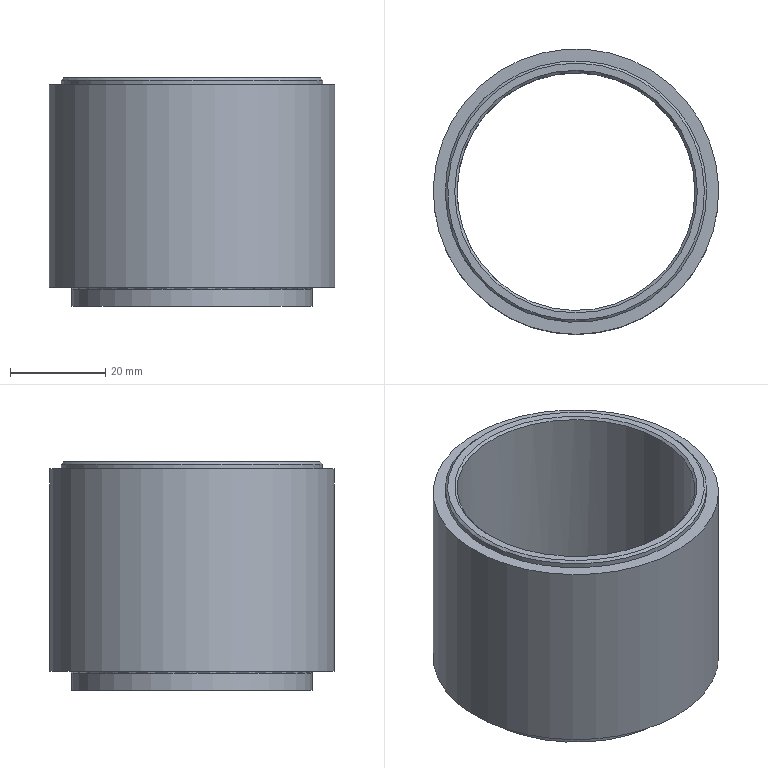Part | STEP file | 1 solid | 11 faces | box 60 x 60 x 48 mm | volume 37487 mm3 | plane 4 | cylinder 4 | cone 2 | torus 1 | commonest cylinder face diameters 50 x1 50.6 x1 54.97 x1 60 x1
STEP:
#1=CARTESIAN_POINT('',(23.383,13.5,31.69));
#2=VERTEX_POINT('',#1);
#3=CARTESIAN_POINT('',(0.,0.,31.69));
#4=DIRECTION('',(0.,0.,1.));
#5=DIRECTION('',(-0.866,0.5,0.));
#6=AXIS2_PLACEMENT_3D('',#3,#4,#5);
#7=CIRCLE('',#6,27.);
#8=EDGE_CURVE('',#2,#2,#7,.T.);
#9=ORIENTED_EDGE('',*,*,#8,.T.);
#10=EDGE_LOOP('',(#9));
#11=FACE_BOUND('',#10,.T.);
#12=CARTESIAN_POINT('',(22.084,12.75,31.69));
#13=VERTEX_POINT('',#12);
#14=CARTESIAN_POINT('',(0.,0.,31.69));
#15=DIRECTION('',(0.,0.,-1.));
#16=DIRECTION('',(0.,-1.,0.));
#17=AXIS2_PLACEMENT_3D('',#14,#15,#16);
#18=CIRCLE('',#17,25.5);
#19=EDGE_CURVE('',#13,#13,#18,.T.);
#20=ORIENTED_EDGE('',*,*,#19,.T.);
#21=EDGE_LOOP('',(#20));
#22=FACE_BOUND('',#21,.T.);
#23=CARTESIAN_POINT('',(0.,0.,31.69));
#24=DIRECTION('',(0.,0.,-1.));
#25=DIRECTION('',(0.,-1.,0.));
#26=AXIS2_PLACEMENT_3D('',#23,#24,#25);
#27=PLANE('',#26);
#28=ADVANCED_FACE('',(#11,#22),#27,.F.);
#29=CARTESIAN_POINT('',(23.803,13.742,31.205));
#30=VERTEX_POINT('',#29);
#31=CARTESIAN_POINT('',(-23.803,-13.742,31.205));
#32=VERTEX_POINT('',#31);
#33=CARTESIAN_POINT('',(0.,0.,31.205));
#34=DIRECTION('',(0.,0.,1.));
#35=DIRECTION('',(0.866,0.5,0.));
#36=AXIS2_PLACEMENT_3D('',#33,#34,#35);
#37=CIRCLE('',#36,27.485);
#38=EDGE_CURVE('',#30,#32,#37,.T.);
#39=ORIENTED_EDGE('',*,*,#38,.T.);
#40=CARTESIAN_POINT('',(0.,0.,31.205));
#41=DIRECTION('',(0.,0.,1.));
#42=DIRECTION('',(-0.866,-0.5,0.));
#43=AXIS2_PLACEMENT_3D('',#40,#41,#42);
#44=CIRCLE('',#43,27.485);
#45=EDGE_CURVE('',#32,#30,#44,.T.);
#46=ORIENTED_EDGE('',*,*,#45,.T.);
#47=EDGE_LOOP('',(#39,#46));
#48=FACE_BOUND('',#47,.T.);
#49=ORIENTED_EDGE('',*,*,#8,.F.);
#50=EDGE_LOOP('',(#49));
#51=FACE_OUTER_BOUND('',#50,.T.);
#52=CARTESIAN_POINT('',(0.,0.,31.447));
#53=DIRECTION('',(0.,0.,-1.));
#54=DIRECTION('',(0.866,0.5,0.));
#55=AXIS2_PLACEMENT_3D('',#52,#53,#54);
#56=CONICAL_SURFACE('',#55,27.243,0.7854);
#57=ADVANCED_FACE('',(#48,#51),#56,.T.);
#58=ORIENTED_EDGE('',*,*,#45,.F.);
#59=ORIENTED_EDGE('',*,*,#38,.F.);
#60=EDGE_LOOP('',(#58,#59));
#61=FACE_BOUND('',#60,.T.);
#62=CARTESIAN_POINT('',(-23.803,-13.742,30.19));
#63=VERTEX_POINT('',#62);
#64=CARTESIAN_POINT('',(0.,0.,30.19));
#65=DIRECTION('',(0.,0.,-1.));
#66=DIRECTION('',(0.866,0.5,0.));
#67=AXIS2_PLACEMENT_3D('',#64,#65,#66);
#68=CIRCLE('',#67,27.485);
#69=EDGE_CURVE('',#63,#63,#68,.T.);
#70=ORIENTED_EDGE('',*,*,#69,.F.);
#71=EDGE_LOOP('',(#70));
#72=FACE_OUTER_BOUND('',#71,.T.);
#73=CARTESIAN_POINT('',(0.,0.,30.115));
#74=DIRECTION('',(0.,0.,-1.));
#75=DIRECTION('',(-0.866,-0.5,0.));
#76=AXIS2_PLACEMENT_3D('',#73,#74,#75);
#77=CYLINDRICAL_SURFACE('',#76,27.485);
#78=ADVANCED_FACE('',(#61,#72),#77,.T.);
#79=CARTESIAN_POINT('',(25.981,15.,30.19));
#80=VERTEX_POINT('',#79);
#81=CARTESIAN_POINT('',(0.,0.,30.19));
#82=DIRECTION('',(0.,0.,1.));
#83=DIRECTION('',(0.866,0.5,0.));
#84=AXIS2_PLACEMENT_3D('',#81,#82,#83);
#85=CIRCLE('',#84,30.);
#86=EDGE_CURVE('',#80,#80,#85,.T.);
#87=ORIENTED_EDGE('',*,*,#86,.T.);
#88=EDGE_LOOP('',(#87));
#89=FACE_BOUND('',#88,.T.);
#90=ORIENTED_EDGE('',*,*,#69,.T.);
#91=EDGE_LOOP('',(#90));
#92=FACE_BOUND('',#91,.T.);
#93=CARTESIAN_POINT('',(0.,0.,30.19));
#94=DIRECTION('',(0.,0.,1.));
#95=DIRECTION('',(1.,0.,0.));
#96=AXIS2_PLACEMENT_3D('',#93,#94,#95);
#97=PLANE('',#96);
#98=ADVANCED_FACE('',(#89,#92),#97,.T.);
#99=ORIENTED_EDGE('',*,*,#86,.F.);
#100=EDGE_LOOP('',(#99));
#101=FACE_OUTER_BOUND('',#100,.T.);
#102=CARTESIAN_POINT('',(25.981,15.,-12.31));
#103=VERTEX_POINT('',#102);
#104=CARTESIAN_POINT('',(0.,0.,-12.31));
#105=DIRECTION('',(0.,0.,-1.));
#106=DIRECTION('',(0.866,0.5,0.));
#107=AXIS2_PLACEMENT_3D('',#104,#105,#106);
#108=CIRCLE('',#107,30.);
#109=EDGE_CURVE('',#103,#103,#108,.T.);
#110=ORIENTED_EDGE('',*,*,#109,.F.);
#111=EDGE_LOOP('',(#110));
#112=FACE_OUTER_BOUND('',#111,.T.);
#113=CARTESIAN_POINT('',(0.,0.,34.09));
#114=DIRECTION('',(0.,0.,1.));
#115=DIRECTION('',(-0.866,-0.5,0.));
#116=AXIS2_PLACEMENT_3D('',#113,#114,#115);
#117=CYLINDRICAL_SURFACE('',#116,30.);
#118=ADVANCED_FACE('',(#101,#112),#117,.T.);
#119=ORIENTED_EDGE('',*,*,#109,.T.);
#120=EDGE_LOOP('',(#119));
#121=FACE_BOUND('',#120,.T.);
#122=CARTESIAN_POINT('',(22.257,12.85,-12.31));
#123=VERTEX_POINT('',#122);
#124=CARTESIAN_POINT('',(0.,0.,-12.31));
#125=DIRECTION('',(0.,0.,1.));
#126=DIRECTION('',(0.866,0.5,0.));
#127=AXIS2_PLACEMENT_3D('',#124,#125,#126);
#128=CIRCLE('',#127,25.7);
#129=EDGE_CURVE('',#123,#123,#128,.T.);
#130=ORIENTED_EDGE('',*,*,#129,.T.);
#131=EDGE_LOOP('',(#130));
#132=FACE_BOUND('',#131,.T.);
#133=CARTESIAN_POINT('',(0.,0.,-12.31));
#134=DIRECTION('',(0.,0.,-1.));
#135=DIRECTION('',(0.,-1.,0.));
#136=AXIS2_PLACEMENT_3D('',#133,#134,#135);
#137=PLANE('',#136);
#138=ADVANCED_FACE('',(#121,#132),#137,.T.);
#139=ORIENTED_EDGE('',*,*,#129,.F.);
#140=EDGE_LOOP('',(#139));
#141=FACE_OUTER_BOUND('',#140,.T.);
#142=CARTESIAN_POINT('',(21.91,12.65,-12.71));
#143=VERTEX_POINT('',#142);
#144=CARTESIAN_POINT('',(-21.91,-12.65,-12.71));
#145=VERTEX_POINT('',#144);
#146=CARTESIAN_POINT('',(0.,0.,-12.71));
#147=DIRECTION('',(0.,0.,1.));
#148=DIRECTION('',(0.866,0.5,0.));
#149=AXIS2_PLACEMENT_3D('',#146,#147,#148);
#150=CIRCLE('',#149,25.3);
#151=EDGE_CURVE('',#143,#145,#150,.T.);
#152=ORIENTED_EDGE('',*,*,#151,.T.);
#153=CARTESIAN_POINT('',(0.,0.,-12.71));
#154=DIRECTION('',(0.,0.,1.));
#155=DIRECTION('',(-0.866,-0.5,0.));
#156=AXIS2_PLACEMENT_3D('',#153,#154,#155);
#157=CIRCLE('',#156,25.3);
#158=EDGE_CURVE('',#145,#143,#157,.T.);
#159=ORIENTED_EDGE('',*,*,#158,.T.);
#160=EDGE_LOOP('',(#152,#159));
#161=FACE_BOUND('',#160,.T.);
#162=CARTESIAN_POINT('',(0.,0.,-12.71));
#163=DIRECTION('',(0.,0.,-1.));
#164=DIRECTION('',(0.866,0.5,0.));
#165=AXIS2_PLACEMENT_3D('',#162,#163,#164);
#166=TOROIDAL_SURFACE('',#165,25.7,0.4);
#167=ADVANCED_FACE('',(#141,#161),#166,.F.);
#168=ORIENTED_EDGE('',*,*,#158,.F.);
#169=ORIENTED_EDGE('',*,*,#151,.F.);
#170=EDGE_LOOP('',(#168,#169));
#171=FACE_BOUND('',#170,.T.);
#172=CARTESIAN_POINT('',(-21.91,-12.65,-16.31));
#173=VERTEX_POINT('',#172);
#174=CARTESIAN_POINT('',(0.,0.,-16.31));
#175=DIRECTION('',(0.,0.,-1.));
#176=DIRECTION('',(0.866,0.5,0.));
#177=AXIS2_PLACEMENT_3D('',#174,#175,#176);
#178=CIRCLE('',#177,25.3);
#179=EDGE_CURVE('',#173,#173,#178,.T.);
#180=ORIENTED_EDGE('',*,*,#179,.F.);
#181=EDGE_LOOP('',(#180));
#182=FACE_OUTER_BOUND('',#181,.T.);
#183=CARTESIAN_POINT('',(0.,0.,34.09));
#184=DIRECTION('',(0.,0.,1.));
#185=DIRECTION('',(-0.866,-0.5,0.));
#186=AXIS2_PLACEMENT_3D('',#183,#184,#185);
#187=CYLINDRICAL_SURFACE('',#186,25.3);
#188=ADVANCED_FACE('',(#171,#182),#187,.T.);
#189=ORIENTED_EDGE('',*,*,#179,.T.);
#190=EDGE_LOOP('',(#189));
#191=FACE_BOUND('',#190,.T.);
#192=CARTESIAN_POINT('',(21.651,12.5,-16.31));
#193=VERTEX_POINT('',#192);
#194=CARTESIAN_POINT('',(0.,0.,-16.31));
#195=DIRECTION('',(0.,0.,1.));
#196=DIRECTION('',(0.866,0.5,0.));
#197=AXIS2_PLACEMENT_3D('',#194,#195,#196);
#198=CIRCLE('',#197,25.);
#199=EDGE_CURVE('',#193,#193,#198,.T.);
#200=ORIENTED_EDGE('',*,*,#199,.T.);
#201=EDGE_LOOP('',(#200));
#202=FACE_BOUND('',#201,.T.);
#203=CARTESIAN_POINT('',(0.,0.,-16.31));
#204=DIRECTION('',(0.,0.,-1.));
#205=DIRECTION('',(0.,-1.,0.));
#206=AXIS2_PLACEMENT_3D('',#203,#204,#205);
#207=PLANE('',#206);
#208=ADVANCED_FACE('',(#191,#202),#207,.T.);
#209=CARTESIAN_POINT('',(21.651,12.5,31.19));
#210=VERTEX_POINT('',#209);
#211=CARTESIAN_POINT('',(21.651,12.5,31.19));
#212=CARTESIAN_POINT('',(21.913,12.046,31.19));
#213=CARTESIAN_POINT('',(22.408,11.123,31.19));
#214=CARTESIAN_POINT('',(23.062,9.694,31.19));
#215=CARTESIAN_POINT('',(23.625,8.226,31.19));
#216=CARTESIAN_POINT('',(24.095,6.726,31.19));
#217=CARTESIAN_POINT('',(24.47,5.2,31.19));
#218=CARTESIAN_POINT('',(24.748,3.653,31.19));
#219=CARTESIAN_POINT('',(24.929,2.092,31.19));
#220=CARTESIAN_POINT('',(25.011,0.5219,31.19));
#221=CARTESIAN_POINT('',(24.994,-1.05,31.19));
#222=CARTESIAN_POINT('',(24.879,-2.617,31.19));
#223=CARTESIAN_POINT('',(24.666,-4.175,31.19));
#224=CARTESIAN_POINT('',(24.355,-5.715,31.19));
#225=CARTESIAN_POINT('',(23.948,-7.234,31.19));
#226=CARTESIAN_POINT('',(23.446,-8.723,31.19));
#227=CARTESIAN_POINT('',(22.852,-10.179,31.19));
#228=CARTESIAN_POINT('',(22.168,-11.594,31.19));
#229=CARTESIAN_POINT('',(21.396,-12.963,31.19));
#230=CARTESIAN_POINT('',(20.54,-14.281,31.19));
#231=CARTESIAN_POINT('',(19.602,-15.543,31.19));
#232=CARTESIAN_POINT('',(18.588,-16.743,31.19));
#233=CARTESIAN_POINT('',(17.499,-17.877,31.19));
#234=CARTESIAN_POINT('',(16.342,-18.941,31.19));
#235=CARTESIAN_POINT('',(15.12,-19.93,31.19));
#236=CARTESIAN_POINT('',(13.839,-20.84,31.19));
#237=CARTESIAN_POINT('',(12.503,-21.668,31.19));
#238=CARTESIAN_POINT('',(11.117,-22.41,31.19));
#239=CARTESIAN_POINT('',(9.688,-23.064,31.19));
#240=CARTESIAN_POINT('',(8.22,-23.627,31.19));
#241=CARTESIAN_POINT('',(6.72,-24.097,31.19));
#242=CARTESIAN_POINT('',(5.194,-24.471,31.19));
#243=CARTESIAN_POINT('',(3.647,-24.749,31.19));
#244=CARTESIAN_POINT('',(2.085,-24.929,31.19));
#245=CARTESIAN_POINT('',(0.5157,-25.011,31.19));
#246=CARTESIAN_POINT('',(-1.056,-24.994,31.19));
#247=CARTESIAN_POINT('',(-2.624,-24.879,31.19));
#248=CARTESIAN_POINT('',(-4.181,-24.665,31.19));
#249=CARTESIAN_POINT('',(-5.722,-24.353,31.19));
#250=CARTESIAN_POINT('',(-7.24,-23.946,31.19));
#251=CARTESIAN_POINT('',(-8.729,-23.444,31.19));
#252=CARTESIAN_POINT('',(-10.184,-22.85,31.19));
#253=CARTESIAN_POINT('',(-11.599,-22.165,31.19));
#254=CARTESIAN_POINT('',(-12.968,-21.393,31.19));
#255=CARTESIAN_POINT('',(-14.286,-20.536,31.19));
#256=CARTESIAN_POINT('',(-15.548,-19.598,31.19));
#257=CARTESIAN_POINT('',(-16.748,-18.583,31.19));
#258=CARTESIAN_POINT('',(-17.882,-17.495,31.19));
#259=CARTESIAN_POINT('',(-18.945,-16.337,31.19));
#260=CARTESIAN_POINT('',(-19.934,-15.115,31.19));
#261=CARTESIAN_POINT('',(-20.841,-13.837,31.19));
#262=CARTESIAN_POINT('',(-21.391,-12.95,31.19));
#263=CARTESIAN_POINT('',(-21.651,-12.5,31.19));
#264=CARTESIAN_POINT('',(-21.913,-12.046,31.19));
#265=CARTESIAN_POINT('',(-22.408,-11.123,31.19));
#266=CARTESIAN_POINT('',(-23.062,-9.694,31.19));
#267=CARTESIAN_POINT('',(-23.625,-8.226,31.19));
#268=CARTESIAN_POINT('',(-24.095,-6.726,31.19));
#269=CARTESIAN_POINT('',(-24.47,-5.2,31.19));
#270=CARTESIAN_POINT('',(-24.748,-3.653,31.19));
#271=CARTESIAN_POINT('',(-24.929,-2.092,31.19));
#272=CARTESIAN_POINT('',(-25.011,-0.5219,31.19));
#273=CARTESIAN_POINT('',(-24.994,1.05,31.19));
#274=CARTESIAN_POINT('',(-24.879,2.617,31.19));
#275=CARTESIAN_POINT('',(-24.666,4.175,31.19));
#276=CARTESIAN_POINT('',(-24.355,5.715,31.19));
#277=CARTESIAN_POINT('',(-23.948,7.234,31.19));
#278=CARTESIAN_POINT('',(-23.446,8.723,31.19));
#279=CARTESIAN_POINT('',(-22.852,10.179,31.19));
#280=CARTESIAN_POINT('',(-22.168,11.594,31.19));
#281=CARTESIAN_POINT('',(-21.396,12.963,31.19));
#282=CARTESIAN_POINT('',(-20.54,14.281,31.19));
#283=CARTESIAN_POINT('',(-19.602,15.543,31.19));
#284=CARTESIAN_POINT('',(-18.588,16.743,31.19));
#285=CARTESIAN_POINT('',(-17.499,17.877,31.19));
#286=CARTESIAN_POINT('',(-16.342,18.941,31.19));
#287=CARTESIAN_POINT('',(-15.12,19.93,31.19));
#288=CARTESIAN_POINT('',(-13.839,20.84,31.19));
#289=CARTESIAN_POINT('',(-12.503,21.668,31.19));
#290=CARTESIAN_POINT('',(-11.117,22.41,31.19));
#291=CARTESIAN_POINT('',(-9.688,23.064,31.19));
#292=CARTESIAN_POINT('',(-8.22,23.627,31.19));
#293=CARTESIAN_POINT('',(-6.72,24.097,31.19));
#294=CARTESIAN_POINT('',(-5.194,24.471,31.19));
#295=CARTESIAN_POINT('',(-3.647,24.749,31.19));
#296=CARTESIAN_POINT('',(-2.085,24.929,31.19));
#297=CARTESIAN_POINT('',(-0.5157,25.011,31.19));
#298=CARTESIAN_POINT('',(1.056,24.994,31.19));
#299=CARTESIAN_POINT('',(2.624,24.879,31.19));
#300=CARTESIAN_POINT('',(4.181,24.665,31.19));
#301=CARTESIAN_POINT('',(5.722,24.353,31.19));
#302=CARTESIAN_POINT('',(7.24,23.946,31.19));
#303=CARTESIAN_POINT('',(8.729,23.444,31.19));
#304=CARTESIAN_POINT('',(10.184,22.85,31.19));
#305=CARTESIAN_POINT('',(11.599,22.165,31.19));
#306=CARTESIAN_POINT('',(12.968,21.393,31.19));
#307=CARTESIAN_POINT('',(14.286,20.536,31.19));
#308=CARTESIAN_POINT('',(15.548,19.598,31.19));
#309=CARTESIAN_POINT('',(16.748,18.583,31.19));
#310=CARTESIAN_POINT('',(17.882,17.495,31.19));
#311=CARTESIAN_POINT('',(18.945,16.337,31.19));
#312=CARTESIAN_POINT('',(19.934,15.115,31.19));
#313=CARTESIAN_POINT('',(20.841,13.837,31.19));
#314=CARTESIAN_POINT('',(21.391,12.95,31.19));
#315=CARTESIAN_POINT('',(21.651,12.5,31.19));
#316=B_SPLINE_CURVE_WITH_KNOTS('',3,(#211,#212,#213,#214,#215,#216,#217,#218,#219,#220,#221,#222,#223,#224,#225,#226,#227,#228,#229,#230,#231,#232,#233,#234,#235,#236,#237,#238,#239,#240,#241,#242,#243,#244,#245,#246,#247,#248,#249,#250,#251,#252,#253,#254,#255,#256,#257,#258,#259,#260,#261,#262,#263,#264,#265,#266,#267,#268,#269,#270,#271,#272,#273,#274,#275,#276,#277,#278,#279,#280,#281,#282,#283,#284,#285,#286,#287,#288,#289,#290,#291,#292,#293,#294,#295,#296,#297,#298,#299,#300,#301,#302,#303,#304,#305,#306,#307,#308,#309,#310,#311,#312,#313,#314,#315),.UNSPECIFIED.,.T.,.F.,(4,1,1,1,1,1,1,1,1,1,1,1,1,1,1,1,1,1,1,1,1,1,1,1,1,1,1,1,1,1,1,1,1,1,1,1,1,1,1,1,1,1,1,1,1,1,1,1,1,1,3,1,1,1,1,1,1,1,1,1,1,1,1,1,1,1,1,1,1,1,1,1,1,1,1,1,1,1,1,1,1,1,1,1,1,1,1,1,1,1,1,1,1,1,1,1,1,1,1,1,4),(0.,0.01,0.02,0.03,0.04001,0.05001,0.06001,0.07001,0.08001,0.09001,0.1,0.11,0.12,0.13,0.14,0.15,0.16,0.17,0.18,0.19,0.2,0.21,0.22,0.23,0.24,0.25,0.26,0.27,0.28,0.29,0.3,0.31,0.3201,0.3301,0.3401,0.3501,0.3601,0.3701,0.3801,0.3901,0.4001,0.4101,0.4201,0.4301,0.4401,0.4501,0.4601,0.4701,0.4801,0.4901,0.5,0.51,0.52,0.53,0.54,0.55,0.56,0.57,0.58,0.59,0.6,0.61,0.62,0.63,0.64,0.65,0.66,0.67,0.68,0.69,0.7,0.71,0.72,0.73,0.74,0.75,0.76,0.77,0.78,0.79,0.8,0.81,0.8201,0.8301,0.8401,0.8501,0.8601,0.8701,0.8801,0.8901,0.9001,0.9101,0.9201,0.9301,0.9401,0.9501,0.9601,0.9701,0.9801,0.9901,1.),.UNSPECIFIED.);
#317=EDGE_CURVE('',#210,#210,#316,.T.);
#318=ORIENTED_EDGE('',*,*,#317,.F.);
#319=EDGE_LOOP('',(#318));
#320=FACE_OUTER_BOUND('',#319,.T.);
#321=ORIENTED_EDGE('',*,*,#199,.F.);
#322=EDGE_LOOP('',(#321));
#323=FACE_OUTER_BOUND('',#322,.T.);
#324=CARTESIAN_POINT('',(0.,0.,34.09));
#325=DIRECTION('',(0.,0.,1.));
#326=DIRECTION('',(-0.866,-0.5,0.));
#327=AXIS2_PLACEMENT_3D('',#324,#325,#326);
#328=CYLINDRICAL_SURFACE('',#327,25.);
#329=ADVANCED_FACE('',(#320,#323),#328,.F.);
#330=ORIENTED_EDGE('',*,*,#19,.F.);
#331=EDGE_LOOP('',(#330));
#332=FACE_OUTER_BOUND('',#331,.T.);
#333=ORIENTED_EDGE('',*,*,#317,.T.);
#334=EDGE_LOOP('',(#333));
#335=FACE_OUTER_BOUND('',#334,.T.);
#336=CARTESIAN_POINT('',(0.,0.,31.44));
#337=DIRECTION('',(0.,0.,1.));
#338=DIRECTION('',(0.866,0.5,0.));
#339=AXIS2_PLACEMENT_3D('',#336,#337,#338);
#340=CONICAL_SURFACE('',#339,25.25,0.7854);
#341=ADVANCED_FACE('',(#332,#335),#340,.F.);
#342=CLOSED_SHELL('',(#28,#57,#78,#98,#118,#138,#167,#188,#208,#329,#341));
#343=MANIFOLD_SOLID_BREP('',#342);
#344=(LENGTH_UNIT()NAMED_UNIT(*)SI_UNIT(.MILLI.,.METRE.));
#345=UNCERTAINTY_MEASURE_WITH_UNIT(LENGTH_MEASURE(0.00001),#344,'','');
#346=(NAMED_UNIT(*)PLANE_ANGLE_UNIT()SI_UNIT($,.RADIAN.));
#347=(NAMED_UNIT(*)SI_UNIT($,.STERADIAN.)SOLID_ANGLE_UNIT());
#348=(GEOMETRIC_REPRESENTATION_CONTEXT(3)GLOBAL_UNCERTAINTY_ASSIGNED_CONTEXT((#345))GLOBAL_UNIT_ASSIGNED_CONTEXT((#344,#346,#347))REPRESENTATION_CONTEXT('',''));
#349=ADVANCED_BREP_SHAPE_REPRESENTATION('',(#343),#348);